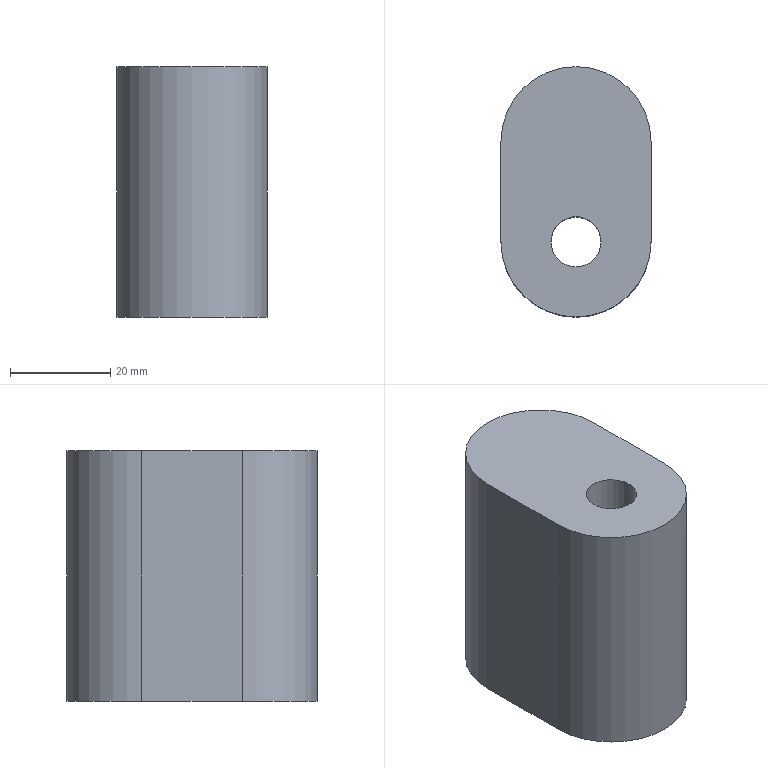Part | NX | features solid 2 | 1 solid | 7 faces | box 30 x 50 x 50 mm | volume 61416 mm3 | plane 4 | cylinder 3 | commonest cylinder face diameters 30 x2 10 x1
STEP:
#1=CARTESIAN_POINT('',(925.,20.,5.));
#2=VERTEX_POINT('',#1);
#3=CARTESIAN_POINT('',(925.,0.,5.));
#4=VERTEX_POINT('',#3);
#5=CARTESIAN_POINT('',(925.,20.,5.));
#6=DIRECTION('',(0.,-1.,0.));
#7=VECTOR('',#6,1000.);
#8=LINE('',#5,#7);
#9=EDGE_CURVE('',#2,#4,#8,.T.);
#10=ORIENTED_EDGE('',*,*,#9,.F.);
#11=CARTESIAN_POINT('',(925.,20.,-45.));
#12=VERTEX_POINT('',#11);
#13=CARTESIAN_POINT('',(925.,20.,-45.));
#14=DIRECTION('',(0.,0.,1.));
#15=VECTOR('',#14,1000.);
#16=LINE('',#13,#15);
#17=EDGE_CURVE('',#12,#2,#16,.T.);
#18=ORIENTED_EDGE('',*,*,#17,.F.);
#19=CARTESIAN_POINT('',(925.,0.,-45.));
#20=VERTEX_POINT('',#19);
#21=CARTESIAN_POINT('',(925.,20.,-45.));
#22=DIRECTION('',(0.,-1.,0.));
#23=VECTOR('',#22,1000.);
#24=LINE('',#21,#23);
#25=EDGE_CURVE('',#12,#20,#24,.T.);
#26=ORIENTED_EDGE('',*,*,#25,.T.);
#27=CARTESIAN_POINT('',(925.,0.,-45.));
#28=DIRECTION('',(0.,0.,1.));
#29=VECTOR('',#28,1000.);
#30=LINE('',#27,#29);
#31=EDGE_CURVE('',#20,#4,#30,.T.);
#32=ORIENTED_EDGE('',*,*,#31,.T.);
#33=EDGE_LOOP('',(#10,#18,#26,#32));
#34=FACE_BOUND('',#33,.T.);
#35=CARTESIAN_POINT('',(925.,20.,-45.));
#36=DIRECTION('',(-1.,0.,0.));
#37=DIRECTION('',(0.,-1.,0.));
#38=AXIS2_PLACEMENT_3D('',#35,#36,#37);
#39=PLANE('',#38);
#40=ADVANCED_FACE('',(#34),#39,.T.);
#41=CARTESIAN_POINT('',(955.,0.,5.));
#42=VERTEX_POINT('',#41);
#43=CARTESIAN_POINT('',(940.,0.,5.));
#44=DIRECTION('',(0.,0.,-1.));
#45=DIRECTION('',(0.,1.,0.));
#46=AXIS2_PLACEMENT_3D('',#43,#44,#45);
#47=CIRCLE('',#46,15.);
#48=EDGE_CURVE('',#42,#4,#47,.T.);
#49=ORIENTED_EDGE('',*,*,#48,.T.);
#50=ORIENTED_EDGE('',*,*,#31,.F.);
#51=CARTESIAN_POINT('',(955.,0.,-45.));
#52=VERTEX_POINT('',#51);
#53=CARTESIAN_POINT('',(940.,0.,-45.));
#54=DIRECTION('',(0.,0.,-1.));
#55=DIRECTION('',(0.,1.,0.));
#56=AXIS2_PLACEMENT_3D('',#53,#54,#55);
#57=CIRCLE('',#56,15.);
#58=EDGE_CURVE('',#52,#20,#57,.T.);
#59=ORIENTED_EDGE('',*,*,#58,.F.);
#60=CARTESIAN_POINT('',(955.,0.,-45.));
#61=DIRECTION('',(0.,0.,1.));
#62=VECTOR('',#61,1000.);
#63=LINE('',#60,#62);
#64=EDGE_CURVE('',#52,#42,#63,.T.);
#65=ORIENTED_EDGE('',*,*,#64,.T.);
#66=EDGE_LOOP('',(#49,#50,#59,#65));
#67=FACE_BOUND('',#66,.T.);
#68=CARTESIAN_POINT('',(940.,0.,-45.));
#69=DIRECTION('',(0.,0.,1.));
#70=DIRECTION('',(1.,0.,0.));
#71=AXIS2_PLACEMENT_3D('',#68,#69,#70);
#72=CYLINDRICAL_SURFACE('',#71,15.);
#73=ADVANCED_FACE('',(#67),#72,.T.);
#74=CARTESIAN_POINT('',(955.,20.,5.));
#75=VERTEX_POINT('',#74);
#76=CARTESIAN_POINT('',(955.,0.,5.));
#77=DIRECTION('',(0.,1.,0.));
#78=VECTOR('',#77,1000.);
#79=LINE('',#76,#78);
#80=EDGE_CURVE('',#42,#75,#79,.T.);
#81=ORIENTED_EDGE('',*,*,#80,.F.);
#82=ORIENTED_EDGE('',*,*,#64,.F.);
#83=CARTESIAN_POINT('',(955.,20.,-45.));
#84=VERTEX_POINT('',#83);
#85=CARTESIAN_POINT('',(955.,0.,-45.));
#86=DIRECTION('',(0.,1.,0.));
#87=VECTOR('',#86,1000.);
#88=LINE('',#85,#87);
#89=EDGE_CURVE('',#52,#84,#88,.T.);
#90=ORIENTED_EDGE('',*,*,#89,.T.);
#91=CARTESIAN_POINT('',(955.,20.,-45.));
#92=DIRECTION('',(0.,0.,1.));
#93=VECTOR('',#92,1000.);
#94=LINE('',#91,#93);
#95=EDGE_CURVE('',#84,#75,#94,.T.);
#96=ORIENTED_EDGE('',*,*,#95,.T.);
#97=EDGE_LOOP('',(#81,#82,#90,#96));
#98=FACE_BOUND('',#97,.T.);
#99=CARTESIAN_POINT('',(955.,0.,-45.));
#100=DIRECTION('',(1.,0.,0.));
#101=DIRECTION('',(0.,0.,-1.));
#102=AXIS2_PLACEMENT_3D('',#99,#100,#101);
#103=PLANE('',#102);
#104=ADVANCED_FACE('',(#98),#103,.T.);
#105=CARTESIAN_POINT('',(940.,20.,5.));
#106=DIRECTION('',(0.,0.,-1.));
#107=DIRECTION('',(0.,1.,0.));
#108=AXIS2_PLACEMENT_3D('',#105,#106,#107);
#109=CIRCLE('',#108,15.);
#110=EDGE_CURVE('',#2,#75,#109,.T.);
#111=ORIENTED_EDGE('',*,*,#110,.T.);
#112=ORIENTED_EDGE('',*,*,#95,.F.);
#113=CARTESIAN_POINT('',(940.,20.,-45.));
#114=DIRECTION('',(0.,0.,-1.));
#115=DIRECTION('',(0.,1.,0.));
#116=AXIS2_PLACEMENT_3D('',#113,#114,#115);
#117=CIRCLE('',#116,15.);
#118=EDGE_CURVE('',#12,#84,#117,.T.);
#119=ORIENTED_EDGE('',*,*,#118,.F.);
#120=ORIENTED_EDGE('',*,*,#17,.T.);
#121=EDGE_LOOP('',(#111,#112,#119,#120));
#122=FACE_BOUND('',#121,.T.);
#123=CARTESIAN_POINT('',(940.,20.,-45.));
#124=DIRECTION('',(0.,0.,1.));
#125=DIRECTION('',(1.,0.,0.));
#126=AXIS2_PLACEMENT_3D('',#123,#124,#125);
#127=CYLINDRICAL_SURFACE('',#126,15.);
#128=ADVANCED_FACE('',(#122),#127,.T.);
#129=CARTESIAN_POINT('',(945.,0.,-45.));
#130=VERTEX_POINT('',#129);
#131=CARTESIAN_POINT('',(940.,0.,-45.));
#132=DIRECTION('',(0.,0.,1.));
#133=DIRECTION('',(1.,0.,0.));
#134=AXIS2_PLACEMENT_3D('',#131,#132,#133);
#135=CIRCLE('',#134,5.);
#136=EDGE_CURVE('',#130,#130,#135,.F.);
#137=ORIENTED_EDGE('',*,*,#136,.T.);
#138=EDGE_LOOP('',(#137));
#139=FACE_BOUND('',#138,.T.);
#140=CARTESIAN_POINT('',(945.,0.,5.));
#141=VERTEX_POINT('',#140);
#142=CARTESIAN_POINT('',(940.,0.,5.));
#143=DIRECTION('',(0.,0.,1.));
#144=DIRECTION('',(1.,0.,0.));
#145=AXIS2_PLACEMENT_3D('',#142,#143,#144);
#146=CIRCLE('',#145,5.);
#147=EDGE_CURVE('',#141,#141,#146,.F.);
#148=ORIENTED_EDGE('',*,*,#147,.F.);
#149=EDGE_LOOP('',(#148));
#150=FACE_BOUND('',#149,.T.);
#151=CARTESIAN_POINT('',(940.,0.,-45.));
#152=DIRECTION('',(0.,0.,1.));
#153=DIRECTION('',(1.,0.,0.));
#154=AXIS2_PLACEMENT_3D('',#151,#152,#153);
#155=CYLINDRICAL_SURFACE('',#154,5.);
#156=ADVANCED_FACE('',(#139,#150),#155,.F.);
#157=ORIENTED_EDGE('',*,*,#25,.F.);
#158=ORIENTED_EDGE('',*,*,#118,.T.);
#159=ORIENTED_EDGE('',*,*,#89,.F.);
#160=ORIENTED_EDGE('',*,*,#58,.T.);
#161=EDGE_LOOP('',(#157,#158,#159,#160));
#162=FACE_BOUND('',#161,.T.);
#163=ORIENTED_EDGE('',*,*,#136,.F.);
#164=EDGE_LOOP('',(#163));
#165=FACE_BOUND('',#164,.T.);
#166=CARTESIAN_POINT('',(940.,0.,-45.));
#167=DIRECTION('',(0.,0.,1.));
#168=DIRECTION('',(0.,1.,0.));
#169=AXIS2_PLACEMENT_3D('',#166,#167,#168);
#170=PLANE('',#169);
#171=ADVANCED_FACE('',(#162,#165),#170,.F.);
#172=ORIENTED_EDGE('',*,*,#9,.T.);
#173=ORIENTED_EDGE('',*,*,#48,.F.);
#174=ORIENTED_EDGE('',*,*,#80,.T.);
#175=ORIENTED_EDGE('',*,*,#110,.F.);
#176=EDGE_LOOP('',(#172,#173,#174,#175));
#177=FACE_BOUND('',#176,.T.);
#178=ORIENTED_EDGE('',*,*,#147,.T.);
#179=EDGE_LOOP('',(#178));
#180=FACE_BOUND('',#179,.T.);
#181=CARTESIAN_POINT('',(940.,0.,5.));
#182=DIRECTION('',(0.,0.,1.));
#183=DIRECTION('',(0.,1.,0.));
#184=AXIS2_PLACEMENT_3D('',#181,#182,#183);
#185=PLANE('',#184);
#186=ADVANCED_FACE('',(#177,#180),#185,.T.);
#187=CLOSED_SHELL('',(#40,#73,#104,#128,#156,#171,#186));
#188=MANIFOLD_SOLID_BREP('',#187);
#189=(LENGTH_UNIT()NAMED_UNIT(*)SI_UNIT(.MILLI.,.METRE.));
#190=UNCERTAINTY_MEASURE_WITH_UNIT(LENGTH_MEASURE(0.00001),#189,'','');
#191=(NAMED_UNIT(*)PLANE_ANGLE_UNIT()SI_UNIT($,.RADIAN.));
#192=(NAMED_UNIT(*)SI_UNIT($,.STERADIAN.)SOLID_ANGLE_UNIT());
#193=(GEOMETRIC_REPRESENTATION_CONTEXT(3)GLOBAL_UNCERTAINTY_ASSIGNED_CONTEXT((#190))GLOBAL_UNIT_ASSIGNED_CONTEXT((#189,#191,#192))REPRESENTATION_CONTEXT('',''));
#194=ADVANCED_BREP_SHAPE_REPRESENTATION('',(#188),#193);